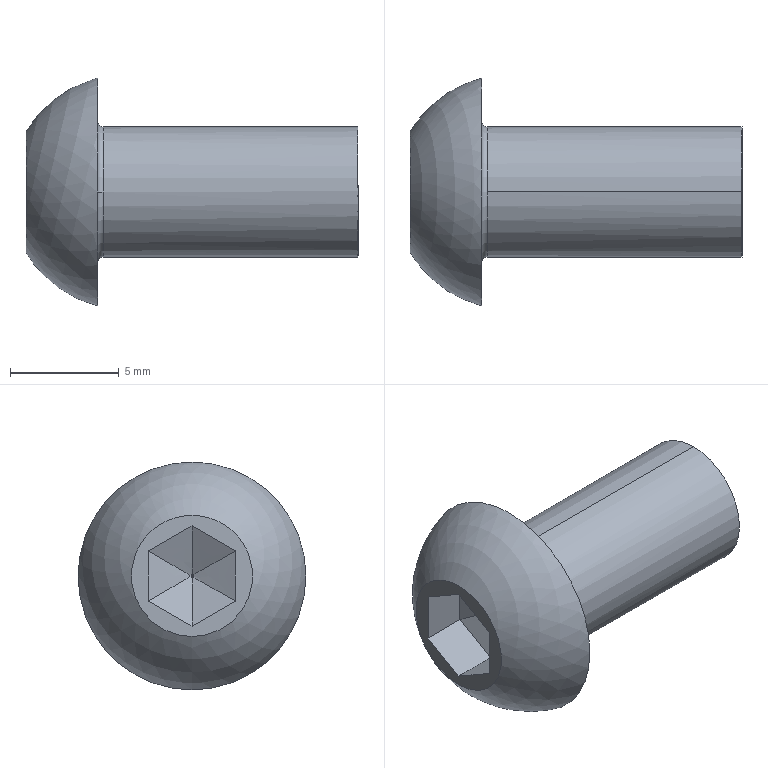Part | SolidWorks | features BaseBody 1 | 1 solid | 21 faces | box 15.3 x 10.5 x 10.5 mm | volume 508.032 mm3 | plane 10 | spline 6 | torus 2 | cylinder 2 | sphere 1 | commonest cylinder face diameters 6 x2